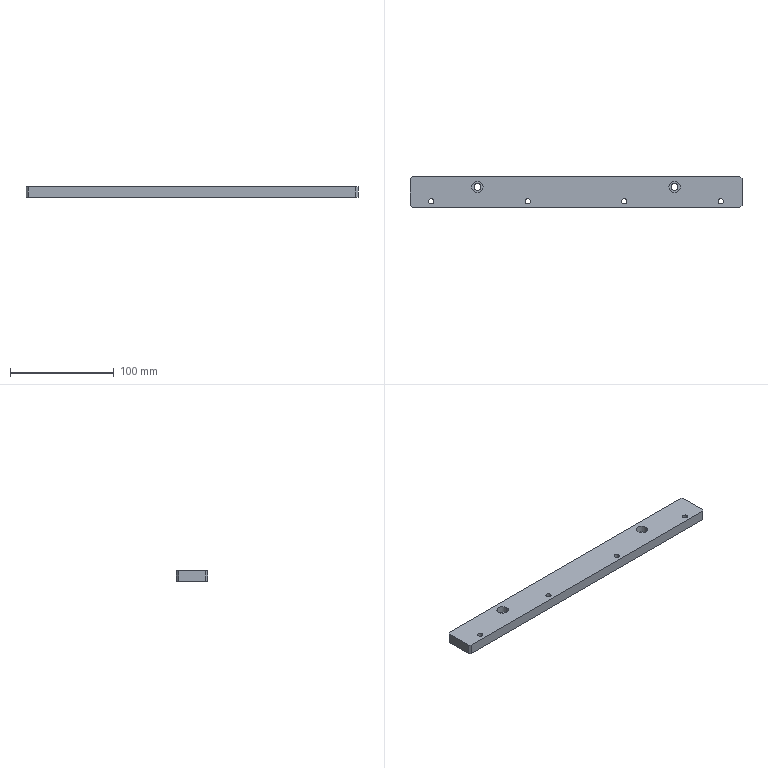Part | SolidWorks | features HoleWzd 2, Chamfer 1, Extrusion 1 | 1 solid | 28 faces | box 320 x 30 x 10 mm | volume 93623 mm3 | cylinder 16 | plane 12 | commonest cylinder face diameters 5 x8 6.6 x4 11 x4
STEP:
#1=CARTESIAN_POINT('',(-100.5,5.,3.2));
#2=VERTEX_POINT('',#1);
#3=CARTESIAN_POINT('',(-89.5,5.,3.2));
#4=VERTEX_POINT('',#3);
#5=CARTESIAN_POINT('',(-95.,5.,3.2));
#6=DIRECTION('',(0.,0.,1.));
#7=DIRECTION('',(1.,0.,0.));
#8=AXIS2_PLACEMENT_3D('',#5,#6,#7);
#9=CIRCLE('',#8,5.5);
#10=EDGE_CURVE('',#2,#4,#9,.T.);
#11=ORIENTED_EDGE('',*,*,#10,.F.);
#12=CARTESIAN_POINT('',(-100.5,5.,10.));
#13=VERTEX_POINT('',#12);
#14=CARTESIAN_POINT('',(-100.5,5.,10.));
#15=DIRECTION('',(0.,0.,1.));
#16=VECTOR('',#15,1000.);
#17=LINE('',#14,#16);
#18=EDGE_CURVE('',#2,#13,#17,.T.);
#19=ORIENTED_EDGE('',*,*,#18,.T.);
#20=CARTESIAN_POINT('',(-89.5,5.,10.));
#21=VERTEX_POINT('',#20);
#22=CARTESIAN_POINT('',(-95.,5.,10.));
#23=DIRECTION('',(0.,0.,1.));
#24=DIRECTION('',(1.,0.,0.));
#25=AXIS2_PLACEMENT_3D('',#22,#23,#24);
#26=CIRCLE('',#25,5.5);
#27=EDGE_CURVE('',#13,#21,#26,.T.);
#28=ORIENTED_EDGE('',*,*,#27,.T.);
#29=CARTESIAN_POINT('',(-89.5,5.,10.));
#30=DIRECTION('',(0.,0.,1.));
#31=VECTOR('',#30,1000.);
#32=LINE('',#29,#31);
#33=EDGE_CURVE('',#4,#21,#32,.T.);
#34=ORIENTED_EDGE('',*,*,#33,.F.);
#35=EDGE_LOOP('',(#11,#19,#28,#34));
#36=FACE_OUTER_BOUND('',#35,.T.);
#37=CARTESIAN_POINT('',(-95.,5.,10.));
#38=DIRECTION('',(0.,0.,1.));
#39=DIRECTION('',(1.,0.,0.));
#40=AXIS2_PLACEMENT_3D('',#37,#38,#39);
#41=CYLINDRICAL_SURFACE('',#40,5.5);
#42=ADVANCED_FACE('',(#36),#41,.F.);
#43=CARTESIAN_POINT('',(-98.3,5.,0.));
#44=VERTEX_POINT('',#43);
#45=CARTESIAN_POINT('',(-91.7,5.,0.));
#46=VERTEX_POINT('',#45);
#47=CARTESIAN_POINT('',(-95.,5.,0.));
#48=DIRECTION('',(0.,0.,1.));
#49=DIRECTION('',(1.,0.,0.));
#50=AXIS2_PLACEMENT_3D('',#47,#48,#49);
#51=CIRCLE('',#50,3.3);
#52=EDGE_CURVE('',#44,#46,#51,.T.);
#53=ORIENTED_EDGE('',*,*,#52,.F.);
#54=CARTESIAN_POINT('',(-98.3,5.,3.2));
#55=VERTEX_POINT('',#54);
#56=CARTESIAN_POINT('',(-98.3,5.,10.));
#57=DIRECTION('',(0.,0.,1.));
#58=VECTOR('',#57,1000.);
#59=LINE('',#56,#58);
#60=EDGE_CURVE('',#44,#55,#59,.T.);
#61=ORIENTED_EDGE('',*,*,#60,.T.);
#62=CARTESIAN_POINT('',(-91.7,5.,3.2));
#63=VERTEX_POINT('',#62);
#64=CARTESIAN_POINT('',(-95.,5.,3.2));
#65=DIRECTION('',(0.,0.,1.));
#66=DIRECTION('',(1.,0.,0.));
#67=AXIS2_PLACEMENT_3D('',#64,#65,#66);
#68=CIRCLE('',#67,3.3);
#69=EDGE_CURVE('',#55,#63,#68,.T.);
#70=ORIENTED_EDGE('',*,*,#69,.T.);
#71=CARTESIAN_POINT('',(-91.7,5.,10.));
#72=DIRECTION('',(0.,0.,1.));
#73=VECTOR('',#72,1000.);
#74=LINE('',#71,#73);
#75=EDGE_CURVE('',#46,#63,#74,.T.);
#76=ORIENTED_EDGE('',*,*,#75,.F.);
#77=EDGE_LOOP('',(#53,#61,#70,#76));
#78=FACE_OUTER_BOUND('',#77,.T.);
#79=CARTESIAN_POINT('',(-95.,5.,10.));
#80=DIRECTION('',(0.,0.,1.));
#81=DIRECTION('',(1.,0.,0.));
#82=AXIS2_PLACEMENT_3D('',#79,#80,#81);
#83=CYLINDRICAL_SURFACE('',#82,3.3);
#84=ADVANCED_FACE('',(#78),#83,.F.);
#85=CARTESIAN_POINT('',(89.5,5.,3.2));
#86=VERTEX_POINT('',#85);
#87=CARTESIAN_POINT('',(100.5,5.,3.2));
#88=VERTEX_POINT('',#87);
#89=CARTESIAN_POINT('',(95.,5.,3.2));
#90=DIRECTION('',(0.,0.,1.));
#91=DIRECTION('',(1.,0.,0.));
#92=AXIS2_PLACEMENT_3D('',#89,#90,#91);
#93=CIRCLE('',#92,5.5);
#94=EDGE_CURVE('',#86,#88,#93,.T.);
#95=ORIENTED_EDGE('',*,*,#94,.F.);
#96=CARTESIAN_POINT('',(89.5,5.,10.));
#97=VERTEX_POINT('',#96);
#98=CARTESIAN_POINT('',(89.5,5.,10.));
#99=DIRECTION('',(0.,0.,1.));
#100=VECTOR('',#99,1000.);
#101=LINE('',#98,#100);
#102=EDGE_CURVE('',#86,#97,#101,.T.);
#103=ORIENTED_EDGE('',*,*,#102,.T.);
#104=CARTESIAN_POINT('',(100.5,5.,10.));
#105=VERTEX_POINT('',#104);
#106=CARTESIAN_POINT('',(95.,5.,10.));
#107=DIRECTION('',(0.,0.,1.));
#108=DIRECTION('',(1.,0.,0.));
#109=AXIS2_PLACEMENT_3D('',#106,#107,#108);
#110=CIRCLE('',#109,5.5);
#111=EDGE_CURVE('',#97,#105,#110,.T.);
#112=ORIENTED_EDGE('',*,*,#111,.T.);
#113=CARTESIAN_POINT('',(100.5,5.,10.));
#114=DIRECTION('',(0.,0.,1.));
#115=VECTOR('',#114,1000.);
#116=LINE('',#113,#115);
#117=EDGE_CURVE('',#88,#105,#116,.T.);
#118=ORIENTED_EDGE('',*,*,#117,.F.);
#119=EDGE_LOOP('',(#95,#103,#112,#118));
#120=FACE_OUTER_BOUND('',#119,.T.);
#121=CARTESIAN_POINT('',(95.,5.,10.));
#122=DIRECTION('',(0.,0.,1.));
#123=DIRECTION('',(1.,0.,0.));
#124=AXIS2_PLACEMENT_3D('',#121,#122,#123);
#125=CYLINDRICAL_SURFACE('',#124,5.5);
#126=ADVANCED_FACE('',(#120),#125,.F.);
#127=CARTESIAN_POINT('',(91.7,5.,0.));
#128=VERTEX_POINT('',#127);
#129=CARTESIAN_POINT('',(98.3,5.,0.));
#130=VERTEX_POINT('',#129);
#131=CARTESIAN_POINT('',(95.,5.,0.));
#132=DIRECTION('',(0.,0.,1.));
#133=DIRECTION('',(1.,0.,0.));
#134=AXIS2_PLACEMENT_3D('',#131,#132,#133);
#135=CIRCLE('',#134,3.3);
#136=EDGE_CURVE('',#128,#130,#135,.T.);
#137=ORIENTED_EDGE('',*,*,#136,.F.);
#138=CARTESIAN_POINT('',(91.7,5.,3.2));
#139=VERTEX_POINT('',#138);
#140=CARTESIAN_POINT('',(91.7,5.,10.));
#141=DIRECTION('',(0.,0.,1.));
#142=VECTOR('',#141,1000.);
#143=LINE('',#140,#142);
#144=EDGE_CURVE('',#128,#139,#143,.T.);
#145=ORIENTED_EDGE('',*,*,#144,.T.);
#146=CARTESIAN_POINT('',(98.3,5.,3.2));
#147=VERTEX_POINT('',#146);
#148=CARTESIAN_POINT('',(95.,5.,3.2));
#149=DIRECTION('',(0.,0.,1.));
#150=DIRECTION('',(1.,0.,0.));
#151=AXIS2_PLACEMENT_3D('',#148,#149,#150);
#152=CIRCLE('',#151,3.3);
#153=EDGE_CURVE('',#139,#147,#152,.T.);
#154=ORIENTED_EDGE('',*,*,#153,.T.);
#155=CARTESIAN_POINT('',(98.3,5.,10.));
#156=DIRECTION('',(0.,0.,1.));
#157=VECTOR('',#156,1000.);
#158=LINE('',#155,#157);
#159=EDGE_CURVE('',#130,#147,#158,.T.);
#160=ORIENTED_EDGE('',*,*,#159,.F.);
#161=EDGE_LOOP('',(#137,#145,#154,#160));
#162=FACE_OUTER_BOUND('',#161,.T.);
#163=CARTESIAN_POINT('',(95.,5.,10.));
#164=DIRECTION('',(0.,0.,1.));
#165=DIRECTION('',(1.,0.,0.));
#166=AXIS2_PLACEMENT_3D('',#163,#164,#165);
#167=CYLINDRICAL_SURFACE('',#166,3.3);
#168=ADVANCED_FACE('',(#162),#167,.F.);
#169=CARTESIAN_POINT('',(-142.,-9.,0.));
#170=VERTEX_POINT('',#169);
#171=CARTESIAN_POINT('',(-137.,-9.,0.));
#172=VERTEX_POINT('',#171);
#173=CARTESIAN_POINT('',(-139.5,-9.,0.));
#174=DIRECTION('',(0.,0.,1.));
#175=DIRECTION('',(1.,0.,0.));
#176=AXIS2_PLACEMENT_3D('',#173,#174,#175);
#177=CIRCLE('',#176,2.5);
#178=EDGE_CURVE('',#170,#172,#177,.T.);
#179=ORIENTED_EDGE('',*,*,#178,.F.);
#180=CARTESIAN_POINT('',(-142.,-9.,10.));
#181=VERTEX_POINT('',#180);
#182=CARTESIAN_POINT('',(-142.,-9.,10.));
#183=DIRECTION('',(0.,0.,1.));
#184=VECTOR('',#183,1000.);
#185=LINE('',#182,#184);
#186=EDGE_CURVE('',#170,#181,#185,.T.);
#187=ORIENTED_EDGE('',*,*,#186,.T.);
#188=CARTESIAN_POINT('',(-137.,-9.,10.));
#189=VERTEX_POINT('',#188);
#190=CARTESIAN_POINT('',(-139.5,-9.,10.));
#191=DIRECTION('',(0.,0.,1.));
#192=DIRECTION('',(1.,0.,0.));
#193=AXIS2_PLACEMENT_3D('',#190,#191,#192);
#194=CIRCLE('',#193,2.5);
#195=EDGE_CURVE('',#181,#189,#194,.T.);
#196=ORIENTED_EDGE('',*,*,#195,.T.);
#197=CARTESIAN_POINT('',(-137.,-9.,10.));
#198=DIRECTION('',(0.,0.,1.));
#199=VECTOR('',#198,1000.);
#200=LINE('',#197,#199);
#201=EDGE_CURVE('',#172,#189,#200,.T.);
#202=ORIENTED_EDGE('',*,*,#201,.F.);
#203=EDGE_LOOP('',(#179,#187,#196,#202));
#204=FACE_OUTER_BOUND('',#203,.T.);
#205=CARTESIAN_POINT('',(-139.5,-9.,10.));
#206=DIRECTION('',(0.,0.,1.));
#207=DIRECTION('',(1.,0.,0.));
#208=AXIS2_PLACEMENT_3D('',#205,#206,#207);
#209=CYLINDRICAL_SURFACE('',#208,2.5);
#210=ADVANCED_FACE('',(#204),#209,.F.);
#211=CARTESIAN_POINT('',(-49.,-9.,0.));
#212=VERTEX_POINT('',#211);
#213=CARTESIAN_POINT('',(-44.,-9.,0.));
#214=VERTEX_POINT('',#213);
#215=CARTESIAN_POINT('',(-46.5,-9.,0.));
#216=DIRECTION('',(0.,0.,1.));
#217=DIRECTION('',(1.,0.,0.));
#218=AXIS2_PLACEMENT_3D('',#215,#216,#217);
#219=CIRCLE('',#218,2.5);
#220=EDGE_CURVE('',#212,#214,#219,.T.);
#221=ORIENTED_EDGE('',*,*,#220,.F.);
#222=CARTESIAN_POINT('',(-49.,-9.,10.));
#223=VERTEX_POINT('',#222);
#224=CARTESIAN_POINT('',(-49.,-9.,10.));
#225=DIRECTION('',(0.,0.,1.));
#226=VECTOR('',#225,1000.);
#227=LINE('',#224,#226);
#228=EDGE_CURVE('',#212,#223,#227,.T.);
#229=ORIENTED_EDGE('',*,*,#228,.T.);
#230=CARTESIAN_POINT('',(-44.,-9.,10.));
#231=VERTEX_POINT('',#230);
#232=CARTESIAN_POINT('',(-46.5,-9.,10.));
#233=DIRECTION('',(0.,0.,1.));
#234=DIRECTION('',(1.,0.,0.));
#235=AXIS2_PLACEMENT_3D('',#232,#233,#234);
#236=CIRCLE('',#235,2.5);
#237=EDGE_CURVE('',#223,#231,#236,.T.);
#238=ORIENTED_EDGE('',*,*,#237,.T.);
#239=CARTESIAN_POINT('',(-44.,-9.,10.));
#240=DIRECTION('',(0.,0.,1.));
#241=VECTOR('',#240,1000.);
#242=LINE('',#239,#241);
#243=EDGE_CURVE('',#214,#231,#242,.T.);
#244=ORIENTED_EDGE('',*,*,#243,.F.);
#245=EDGE_LOOP('',(#221,#229,#238,#244));
#246=FACE_OUTER_BOUND('',#245,.T.);
#247=CARTESIAN_POINT('',(-46.5,-9.,10.));
#248=DIRECTION('',(0.,0.,1.));
#249=DIRECTION('',(1.,0.,0.));
#250=AXIS2_PLACEMENT_3D('',#247,#248,#249);
#251=CYLINDRICAL_SURFACE('',#250,2.5);
#252=ADVANCED_FACE('',(#246),#251,.F.);
#253=CARTESIAN_POINT('',(44.,-9.,0.));
#254=VERTEX_POINT('',#253);
#255=CARTESIAN_POINT('',(49.,-9.,0.));
#256=VERTEX_POINT('',#255);
#257=CARTESIAN_POINT('',(46.5,-9.,0.));
#258=DIRECTION('',(0.,0.,1.));
#259=DIRECTION('',(1.,0.,0.));
#260=AXIS2_PLACEMENT_3D('',#257,#258,#259);
#261=CIRCLE('',#260,2.5);
#262=EDGE_CURVE('',#254,#256,#261,.T.);
#263=ORIENTED_EDGE('',*,*,#262,.F.);
#264=CARTESIAN_POINT('',(44.,-9.,10.));
#265=VERTEX_POINT('',#264);
#266=CARTESIAN_POINT('',(44.,-9.,10.));
#267=DIRECTION('',(0.,0.,1.));
#268=VECTOR('',#267,1000.);
#269=LINE('',#266,#268);
#270=EDGE_CURVE('',#254,#265,#269,.T.);
#271=ORIENTED_EDGE('',*,*,#270,.T.);
#272=CARTESIAN_POINT('',(49.,-9.,10.));
#273=VERTEX_POINT('',#272);
#274=CARTESIAN_POINT('',(46.5,-9.,10.));
#275=DIRECTION('',(0.,0.,1.));
#276=DIRECTION('',(1.,0.,0.));
#277=AXIS2_PLACEMENT_3D('',#274,#275,#276);
#278=CIRCLE('',#277,2.5);
#279=EDGE_CURVE('',#265,#273,#278,.T.);
#280=ORIENTED_EDGE('',*,*,#279,.T.);
#281=CARTESIAN_POINT('',(49.,-9.,10.));
#282=DIRECTION('',(0.,0.,1.));
#283=VECTOR('',#282,1000.);
#284=LINE('',#281,#283);
#285=EDGE_CURVE('',#256,#273,#284,.T.);
#286=ORIENTED_EDGE('',*,*,#285,.F.);
#287=EDGE_LOOP('',(#263,#271,#280,#286));
#288=FACE_OUTER_BOUND('',#287,.T.);
#289=CARTESIAN_POINT('',(46.5,-9.,10.));
#290=DIRECTION('',(0.,0.,1.));
#291=DIRECTION('',(1.,0.,0.));
#292=AXIS2_PLACEMENT_3D('',#289,#290,#291);
#293=CYLINDRICAL_SURFACE('',#292,2.5);
#294=ADVANCED_FACE('',(#288),#293,.F.);
#295=CARTESIAN_POINT('',(137.,-9.,0.));
#296=VERTEX_POINT('',#295);
#297=CARTESIAN_POINT('',(142.,-9.,0.));
#298=VERTEX_POINT('',#297);
#299=CARTESIAN_POINT('',(139.5,-9.,0.));
#300=DIRECTION('',(0.,0.,1.));
#301=DIRECTION('',(1.,0.,0.));
#302=AXIS2_PLACEMENT_3D('',#299,#300,#301);
#303=CIRCLE('',#302,2.5);
#304=EDGE_CURVE('',#296,#298,#303,.T.);
#305=ORIENTED_EDGE('',*,*,#304,.F.);
#306=CARTESIAN_POINT('',(137.,-9.,10.));
#307=VERTEX_POINT('',#306);
#308=CARTESIAN_POINT('',(137.,-9.,10.));
#309=DIRECTION('',(0.,0.,1.));
#310=VECTOR('',#309,1000.);
#311=LINE('',#308,#310);
#312=EDGE_CURVE('',#296,#307,#311,.T.);
#313=ORIENTED_EDGE('',*,*,#312,.T.);
#314=CARTESIAN_POINT('',(142.,-9.,10.));
#315=VERTEX_POINT('',#314);
#316=CARTESIAN_POINT('',(139.5,-9.,10.));
#317=DIRECTION('',(0.,0.,1.));
#318=DIRECTION('',(1.,0.,0.));
#319=AXIS2_PLACEMENT_3D('',#316,#317,#318);
#320=CIRCLE('',#319,2.5);
#321=EDGE_CURVE('',#307,#315,#320,.T.);
#322=ORIENTED_EDGE('',*,*,#321,.T.);
#323=CARTESIAN_POINT('',(142.,-9.,10.));
#324=DIRECTION('',(0.,0.,1.));
#325=VECTOR('',#324,1000.);
#326=LINE('',#323,#325);
#327=EDGE_CURVE('',#298,#315,#326,.T.);
#328=ORIENTED_EDGE('',*,*,#327,.F.);
#329=EDGE_LOOP('',(#305,#313,#322,#328));
#330=FACE_OUTER_BOUND('',#329,.T.);
#331=CARTESIAN_POINT('',(139.5,-9.,10.));
#332=DIRECTION('',(0.,0.,1.));
#333=DIRECTION('',(1.,0.,0.));
#334=AXIS2_PLACEMENT_3D('',#331,#332,#333);
#335=CYLINDRICAL_SURFACE('',#334,2.5);
#336=ADVANCED_FACE('',(#330),#335,.F.);
#337=CARTESIAN_POINT('',(160.,-13.,10.));
#338=VERTEX_POINT('',#337);
#339=CARTESIAN_POINT('',(160.,13.,10.));
#340=VERTEX_POINT('',#339);
#341=CARTESIAN_POINT('',(160.,-15.,10.));
#342=DIRECTION('',(0.,1.,0.));
#343=VECTOR('',#342,1000.);
#344=LINE('',#341,#343);
#345=EDGE_CURVE('',#338,#340,#344,.T.);
#346=ORIENTED_EDGE('',*,*,#345,.F.);
#347=CARTESIAN_POINT('',(160.,-13.,0.));
#348=VERTEX_POINT('',#347);
#349=CARTESIAN_POINT('',(160.,-13.,10.));
#350=DIRECTION('',(0.,0.,-1.));
#351=VECTOR('',#350,1000.);
#352=LINE('',#349,#351);
#353=EDGE_CURVE('',#338,#348,#352,.T.);
#354=ORIENTED_EDGE('',*,*,#353,.T.);
#355=CARTESIAN_POINT('',(160.,13.,0.));
#356=VERTEX_POINT('',#355);
#357=CARTESIAN_POINT('',(160.,-15.,0.));
#358=DIRECTION('',(0.,1.,0.));
#359=VECTOR('',#358,1000.);
#360=LINE('',#357,#359);
#361=EDGE_CURVE('',#348,#356,#360,.T.);
#362=ORIENTED_EDGE('',*,*,#361,.T.);
#363=CARTESIAN_POINT('',(160.,13.,10.));
#364=DIRECTION('',(0.,0.,1.));
#365=VECTOR('',#364,1000.);
#366=LINE('',#363,#365);
#367=EDGE_CURVE('',#356,#340,#366,.T.);
#368=ORIENTED_EDGE('',*,*,#367,.T.);
#369=EDGE_LOOP('',(#346,#354,#362,#368));
#370=FACE_OUTER_BOUND('',#369,.T.);
#371=CARTESIAN_POINT('',(160.,-15.,10.));
#372=DIRECTION('',(-1.,0.,0.));
#373=DIRECTION('',(0.,0.,1.));
#374=AXIS2_PLACEMENT_3D('',#371,#372,#373);
#375=PLANE('',#374);
#376=ADVANCED_FACE('',(#370),#375,.F.);
#377=CARTESIAN_POINT('',(158.,15.,10.));
#378=VERTEX_POINT('',#377);
#379=CARTESIAN_POINT('',(-158.,15.,10.));
#380=VERTEX_POINT('',#379);
#381=CARTESIAN_POINT('',(-160.,15.,10.));
#382=DIRECTION('',(-1.,0.,0.));
#383=VECTOR('',#382,1000.);
#384=LINE('',#381,#383);
#385=EDGE_CURVE('',#378,#380,#384,.T.);
#386=ORIENTED_EDGE('',*,*,#385,.F.);
#387=CARTESIAN_POINT('',(158.,15.,0.));
#388=VERTEX_POINT('',#387);
#389=CARTESIAN_POINT('',(158.,15.,10.));
#390=DIRECTION('',(0.,0.,-1.));
#391=VECTOR('',#390,1000.);
#392=LINE('',#389,#391);
#393=EDGE_CURVE('',#378,#388,#392,.T.);
#394=ORIENTED_EDGE('',*,*,#393,.T.);
#395=CARTESIAN_POINT('',(-158.,15.,0.));
#396=VERTEX_POINT('',#395);
#397=CARTESIAN_POINT('',(-160.,15.,0.));
#398=DIRECTION('',(-1.,0.,0.));
#399=VECTOR('',#398,1000.);
#400=LINE('',#397,#399);
#401=EDGE_CURVE('',#388,#396,#400,.T.);
#402=ORIENTED_EDGE('',*,*,#401,.T.);
#403=CARTESIAN_POINT('',(-158.,15.,10.));
#404=DIRECTION('',(0.,0.,1.));
#405=VECTOR('',#404,1000.);
#406=LINE('',#403,#405);
#407=EDGE_CURVE('',#396,#380,#406,.T.);
#408=ORIENTED_EDGE('',*,*,#407,.T.);
#409=EDGE_LOOP('',(#386,#394,#402,#408));
#410=FACE_OUTER_BOUND('',#409,.T.);
#411=CARTESIAN_POINT('',(-160.,15.,10.));
#412=DIRECTION('',(0.,-1.,0.));
#413=DIRECTION('',(0.,0.,-1.));
#414=AXIS2_PLACEMENT_3D('',#411,#412,#413);
#415=PLANE('',#414);
#416=ADVANCED_FACE('',(#410),#415,.F.);
#417=CARTESIAN_POINT('',(-160.,13.,0.));
#418=VERTEX_POINT('',#417);
#419=CARTESIAN_POINT('',(-160.,-13.,0.));
#420=VERTEX_POINT('',#419);
#421=CARTESIAN_POINT('',(-160.,-15.,0.));
#422=DIRECTION('',(0.,-1.,0.));
#423=VECTOR('',#422,1000.);
#424=LINE('',#421,#423);
#425=EDGE_CURVE('',#418,#420,#424,.T.);
#426=ORIENTED_EDGE('',*,*,#425,.T.);
#427=CARTESIAN_POINT('',(-160.,-13.,10.));
#428=VERTEX_POINT('',#427);
#429=CARTESIAN_POINT('',(-160.,-13.,10.));
#430=DIRECTION('',(0.,0.,1.));
#431=VECTOR('',#430,1000.);
#432=LINE('',#429,#431);
#433=EDGE_CURVE('',#420,#428,#432,.T.);
#434=ORIENTED_EDGE('',*,*,#433,.T.);
#435=CARTESIAN_POINT('',(-160.,13.,10.));
#436=VERTEX_POINT('',#435);
#437=CARTESIAN_POINT('',(-160.,-15.,10.));
#438=DIRECTION('',(0.,-1.,0.));
#439=VECTOR('',#438,1000.);
#440=LINE('',#437,#439);
#441=EDGE_CURVE('',#436,#428,#440,.T.);
#442=ORIENTED_EDGE('',*,*,#441,.F.);
#443=CARTESIAN_POINT('',(-160.,13.,10.));
#444=DIRECTION('',(0.,0.,-1.));
#445=VECTOR('',#444,1000.);
#446=LINE('',#443,#445);
#447=EDGE_CURVE('',#436,#418,#446,.T.);
#448=ORIENTED_EDGE('',*,*,#447,.T.);
#449=EDGE_LOOP('',(#426,#434,#442,#448));
#450=FACE_OUTER_BOUND('',#449,.T.);
#451=CARTESIAN_POINT('',(-160.,-15.,10.));
#452=DIRECTION('',(1.,0.,0.));
#453=DIRECTION('',(0.,0.,-1.));
#454=AXIS2_PLACEMENT_3D('',#451,#452,#453);
#455=PLANE('',#454);
#456=ADVANCED_FACE('',(#450),#455,.F.);
#457=CARTESIAN_POINT('',(-158.,-15.,0.));
#458=VERTEX_POINT('',#457);
#459=CARTESIAN_POINT('',(158.,-15.,0.));
#460=VERTEX_POINT('',#459);
#461=CARTESIAN_POINT('',(-160.,-15.,0.));
#462=DIRECTION('',(1.,0.,0.));
#463=VECTOR('',#462,1000.);
#464=LINE('',#461,#463);
#465=EDGE_CURVE('',#458,#460,#464,.T.);
#466=ORIENTED_EDGE('',*,*,#465,.T.);
#467=CARTESIAN_POINT('',(158.,-15.,10.));
#468=VERTEX_POINT('',#467);
#469=CARTESIAN_POINT('',(158.,-15.,10.));
#470=DIRECTION('',(0.,0.,1.));
#471=VECTOR('',#470,1000.);
#472=LINE('',#469,#471);
#473=EDGE_CURVE('',#460,#468,#472,.T.);
#474=ORIENTED_EDGE('',*,*,#473,.T.);
#475=CARTESIAN_POINT('',(-158.,-15.,10.));
#476=VERTEX_POINT('',#475);
#477=CARTESIAN_POINT('',(-160.,-15.,10.));
#478=DIRECTION('',(1.,0.,0.));
#479=VECTOR('',#478,1000.);
#480=LINE('',#477,#479);
#481=EDGE_CURVE('',#476,#468,#480,.T.);
#482=ORIENTED_EDGE('',*,*,#481,.F.);
#483=CARTESIAN_POINT('',(-158.,-15.,10.));
#484=DIRECTION('',(0.,0.,-1.));
#485=VECTOR('',#484,1000.);
#486=LINE('',#483,#485);
#487=EDGE_CURVE('',#476,#458,#486,.T.);
#488=ORIENTED_EDGE('',*,*,#487,.T.);
#489=EDGE_LOOP('',(#466,#474,#482,#488));
#490=FACE_OUTER_BOUND('',#489,.T.);
#491=CARTESIAN_POINT('',(-160.,-15.,10.));
#492=DIRECTION('',(0.,1.,0.));
#493=DIRECTION('',(0.,0.,1.));
#494=AXIS2_PLACEMENT_3D('',#491,#492,#493);
#495=PLANE('',#494);
#496=ADVANCED_FACE('',(#490),#495,.F.);
#497=CARTESIAN_POINT('',(-95.,5.,10.));
#498=DIRECTION('',(0.,0.,1.));
#499=DIRECTION('',(1.,0.,0.));
#500=AXIS2_PLACEMENT_3D('',#497,#498,#499);
#501=CIRCLE('',#500,5.5);
#502=EDGE_CURVE('',#21,#13,#501,.T.);
#503=ORIENTED_EDGE('',*,*,#502,.F.);
#504=ORIENTED_EDGE('',*,*,#27,.F.);
#505=EDGE_LOOP('',(#503,#504));
#506=FACE_BOUND('',#505,.T.);
#507=CARTESIAN_POINT('',(95.,5.,10.));
#508=DIRECTION('',(0.,0.,1.));
#509=DIRECTION('',(1.,0.,0.));
#510=AXIS2_PLACEMENT_3D('',#507,#508,#509);
#511=CIRCLE('',#510,5.5);
#512=EDGE_CURVE('',#105,#97,#511,.T.);
#513=ORIENTED_EDGE('',*,*,#512,.F.);
#514=ORIENTED_EDGE('',*,*,#111,.F.);
#515=EDGE_LOOP('',(#513,#514));
#516=FACE_BOUND('',#515,.T.);
#517=CARTESIAN_POINT('',(-139.5,-9.,10.));
#518=DIRECTION('',(0.,0.,1.));
#519=DIRECTION('',(1.,0.,0.));
#520=AXIS2_PLACEMENT_3D('',#517,#518,#519);
#521=CIRCLE('',#520,2.5);
#522=EDGE_CURVE('',#189,#181,#521,.T.);
#523=ORIENTED_EDGE('',*,*,#522,.F.);
#524=ORIENTED_EDGE('',*,*,#195,.F.);
#525=EDGE_LOOP('',(#523,#524));
#526=FACE_BOUND('',#525,.T.);
#527=CARTESIAN_POINT('',(-46.5,-9.,10.));
#528=DIRECTION('',(0.,0.,1.));
#529=DIRECTION('',(1.,0.,0.));
#530=AXIS2_PLACEMENT_3D('',#527,#528,#529);
#531=CIRCLE('',#530,2.5);
#532=EDGE_CURVE('',#231,#223,#531,.T.);
#533=ORIENTED_EDGE('',*,*,#532,.F.);
#534=ORIENTED_EDGE('',*,*,#237,.F.);
#535=EDGE_LOOP('',(#533,#534));
#536=FACE_BOUND('',#535,.T.);
#537=CARTESIAN_POINT('',(46.5,-9.,10.));
#538=DIRECTION('',(0.,0.,1.));
#539=DIRECTION('',(1.,0.,0.));
#540=AXIS2_PLACEMENT_3D('',#537,#538,#539);
#541=CIRCLE('',#540,2.5);
#542=EDGE_CURVE('',#273,#265,#541,.T.);
#543=ORIENTED_EDGE('',*,*,#542,.F.);
#544=ORIENTED_EDGE('',*,*,#279,.F.);
#545=EDGE_LOOP('',(#543,#544));
#546=FACE_BOUND('',#545,.T.);
#547=CARTESIAN_POINT('',(139.5,-9.,10.));
#548=DIRECTION('',(0.,0.,1.));
#549=DIRECTION('',(1.,0.,0.));
#550=AXIS2_PLACEMENT_3D('',#547,#548,#549);
#551=CIRCLE('',#550,2.5);
#552=EDGE_CURVE('',#315,#307,#551,.T.);
#553=ORIENTED_EDGE('',*,*,#552,.F.);
#554=ORIENTED_EDGE('',*,*,#321,.F.);
#555=EDGE_LOOP('',(#553,#554));
#556=FACE_BOUND('',#555,.T.);
#557=ORIENTED_EDGE('',*,*,#481,.T.);
#558=CARTESIAN_POINT('',(160.,-13.,10.));
#559=DIRECTION('',(0.7071,0.7071,0.));
#560=VECTOR('',#559,1000.);
#561=LINE('',#558,#560);
#562=EDGE_CURVE('',#468,#338,#561,.T.);
#563=ORIENTED_EDGE('',*,*,#562,.T.);
#564=ORIENTED_EDGE('',*,*,#345,.T.);
#565=CARTESIAN_POINT('',(158.,15.,10.));
#566=DIRECTION('',(-0.7071,0.7071,0.));
#567=VECTOR('',#566,1000.);
#568=LINE('',#565,#567);
#569=EDGE_CURVE('',#340,#378,#568,.T.);
#570=ORIENTED_EDGE('',*,*,#569,.T.);
#571=ORIENTED_EDGE('',*,*,#385,.T.);
#572=CARTESIAN_POINT('',(-160.,13.,10.));
#573=DIRECTION('',(-0.7071,-0.7071,0.));
#574=VECTOR('',#573,1000.);
#575=LINE('',#572,#574);
#576=EDGE_CURVE('',#380,#436,#575,.T.);
#577=ORIENTED_EDGE('',*,*,#576,.T.);
#578=ORIENTED_EDGE('',*,*,#441,.T.);
#579=CARTESIAN_POINT('',(-158.,-15.,10.));
#580=DIRECTION('',(0.7071,-0.7071,0.));
#581=VECTOR('',#580,1000.);
#582=LINE('',#579,#581);
#583=EDGE_CURVE('',#428,#476,#582,.T.);
#584=ORIENTED_EDGE('',*,*,#583,.T.);
#585=EDGE_LOOP('',(#557,#563,#564,#570,#571,#577,#578,#584));
#586=FACE_OUTER_BOUND('',#585,.T.);
#587=CARTESIAN_POINT('',(0.,0.,10.));
#588=DIRECTION('',(0.,0.,-1.));
#589=DIRECTION('',(-1.,0.,0.));
#590=AXIS2_PLACEMENT_3D('',#587,#588,#589);
#591=PLANE('',#590);
#592=ADVANCED_FACE('',(#506,#516,#526,#536,#546,#556,#586),#591,.F.);
#593=CARTESIAN_POINT('',(-95.,5.,0.));
#594=DIRECTION('',(0.,0.,1.));
#595=DIRECTION('',(1.,0.,0.));
#596=AXIS2_PLACEMENT_3D('',#593,#594,#595);
#597=CIRCLE('',#596,3.3);
#598=EDGE_CURVE('',#46,#44,#597,.T.);
#599=ORIENTED_EDGE('',*,*,#598,.T.);
#600=ORIENTED_EDGE('',*,*,#52,.T.);
#601=EDGE_LOOP('',(#599,#600));
#602=FACE_BOUND('',#601,.T.);
#603=CARTESIAN_POINT('',(95.,5.,0.));
#604=DIRECTION('',(0.,0.,1.));
#605=DIRECTION('',(1.,0.,0.));
#606=AXIS2_PLACEMENT_3D('',#603,#604,#605);
#607=CIRCLE('',#606,3.3);
#608=EDGE_CURVE('',#130,#128,#607,.T.);
#609=ORIENTED_EDGE('',*,*,#608,.T.);
#610=ORIENTED_EDGE('',*,*,#136,.T.);
#611=EDGE_LOOP('',(#609,#610));
#612=FACE_BOUND('',#611,.T.);
#613=CARTESIAN_POINT('',(-139.5,-9.,0.));
#614=DIRECTION('',(0.,0.,1.));
#615=DIRECTION('',(1.,0.,0.));
#616=AXIS2_PLACEMENT_3D('',#613,#614,#615);
#617=CIRCLE('',#616,2.5);
#618=EDGE_CURVE('',#172,#170,#617,.T.);
#619=ORIENTED_EDGE('',*,*,#618,.T.);
#620=ORIENTED_EDGE('',*,*,#178,.T.);
#621=EDGE_LOOP('',(#619,#620));
#622=FACE_BOUND('',#621,.T.);
#623=CARTESIAN_POINT('',(-46.5,-9.,0.));
#624=DIRECTION('',(0.,0.,1.));
#625=DIRECTION('',(1.,0.,0.));
#626=AXIS2_PLACEMENT_3D('',#623,#624,#625);
#627=CIRCLE('',#626,2.5);
#628=EDGE_CURVE('',#214,#212,#627,.T.);
#629=ORIENTED_EDGE('',*,*,#628,.T.);
#630=ORIENTED_EDGE('',*,*,#220,.T.);
#631=EDGE_LOOP('',(#629,#630));
#632=FACE_BOUND('',#631,.T.);
#633=CARTESIAN_POINT('',(46.5,-9.,0.));
#634=DIRECTION('',(0.,0.,1.));
#635=DIRECTION('',(1.,0.,0.));
#636=AXIS2_PLACEMENT_3D('',#633,#634,#635);
#637=CIRCLE('',#636,2.5);
#638=EDGE_CURVE('',#256,#254,#637,.T.);
#639=ORIENTED_EDGE('',*,*,#638,.T.);
#640=ORIENTED_EDGE('',*,*,#262,.T.);
#641=EDGE_LOOP('',(#639,#640));
#642=FACE_BOUND('',#641,.T.);
#643=CARTESIAN_POINT('',(139.5,-9.,0.));
#644=DIRECTION('',(0.,0.,1.));
#645=DIRECTION('',(1.,0.,0.));
#646=AXIS2_PLACEMENT_3D('',#643,#644,#645);
#647=CIRCLE('',#646,2.5);
#648=EDGE_CURVE('',#298,#296,#647,.T.);
#649=ORIENTED_EDGE('',*,*,#648,.T.);
#650=ORIENTED_EDGE('',*,*,#304,.T.);
#651=EDGE_LOOP('',(#649,#650));
#652=FACE_BOUND('',#651,.T.);
#653=ORIENTED_EDGE('',*,*,#361,.F.);
#654=CARTESIAN_POINT('',(86.5,-86.5,0.));
#655=DIRECTION('',(-0.7071,-0.7071,0.));
#656=VECTOR('',#655,1000.);
#657=LINE('',#654,#656);
#658=EDGE_CURVE('',#348,#460,#657,.T.);
#659=ORIENTED_EDGE('',*,*,#658,.T.);
#660=ORIENTED_EDGE('',*,*,#465,.F.);
#661=CARTESIAN_POINT('',(-86.5,-86.5,0.));
#662=DIRECTION('',(-0.7071,0.7071,0.));
#663=VECTOR('',#662,1000.);
#664=LINE('',#661,#663);
#665=EDGE_CURVE('',#458,#420,#664,.T.);
#666=ORIENTED_EDGE('',*,*,#665,.T.);
#667=ORIENTED_EDGE('',*,*,#425,.F.);
#668=CARTESIAN_POINT('',(-86.5,86.5,0.));
#669=DIRECTION('',(0.7071,0.7071,0.));
#670=VECTOR('',#669,1000.);
#671=LINE('',#668,#670);
#672=EDGE_CURVE('',#418,#396,#671,.T.);
#673=ORIENTED_EDGE('',*,*,#672,.T.);
#674=ORIENTED_EDGE('',*,*,#401,.F.);
#675=CARTESIAN_POINT('',(86.5,86.5,0.));
#676=DIRECTION('',(0.7071,-0.7071,0.));
#677=VECTOR('',#676,1000.);
#678=LINE('',#675,#677);
#679=EDGE_CURVE('',#388,#356,#678,.T.);
#680=ORIENTED_EDGE('',*,*,#679,.T.);
#681=EDGE_LOOP('',(#653,#659,#660,#666,#667,#673,#674,#680));
#682=FACE_OUTER_BOUND('',#681,.T.);
#683=CARTESIAN_POINT('',(0.,0.,0.));
#684=DIRECTION('',(0.,0.,-1.));
#685=DIRECTION('',(-1.,0.,0.));
#686=AXIS2_PLACEMENT_3D('',#683,#684,#685);
#687=PLANE('',#686);
#688=ADVANCED_FACE('',(#602,#612,#622,#632,#642,#652,#682),#687,.T.);
#689=ORIENTED_EDGE('',*,*,#562,.F.);
#690=ORIENTED_EDGE('',*,*,#473,.F.);
#691=ORIENTED_EDGE('',*,*,#658,.F.);
#692=ORIENTED_EDGE('',*,*,#353,.F.);
#693=EDGE_LOOP('',(#689,#690,#691,#692));
#694=FACE_OUTER_BOUND('',#693,.T.);
#695=CARTESIAN_POINT('',(160.,-13.,10.));
#696=DIRECTION('',(-0.7071,0.7071,0.));
#697=DIRECTION('',(0.,0.,-1.));
#698=AXIS2_PLACEMENT_3D('',#695,#696,#697);
#699=PLANE('',#698);
#700=ADVANCED_FACE('',(#694),#699,.F.);
#701=ORIENTED_EDGE('',*,*,#569,.F.);
#702=ORIENTED_EDGE('',*,*,#367,.F.);
#703=ORIENTED_EDGE('',*,*,#679,.F.);
#704=ORIENTED_EDGE('',*,*,#393,.F.);
#705=EDGE_LOOP('',(#701,#702,#703,#704));
#706=FACE_OUTER_BOUND('',#705,.T.);
#707=CARTESIAN_POINT('',(158.,15.,10.));
#708=DIRECTION('',(-0.7071,-0.7071,0.));
#709=DIRECTION('',(0.,0.,-1.));
#710=AXIS2_PLACEMENT_3D('',#707,#708,#709);
#711=PLANE('',#710);
#712=ADVANCED_FACE('',(#706),#711,.F.);
#713=ORIENTED_EDGE('',*,*,#583,.F.);
#714=ORIENTED_EDGE('',*,*,#433,.F.);
#715=ORIENTED_EDGE('',*,*,#665,.F.);
#716=ORIENTED_EDGE('',*,*,#487,.F.);
#717=EDGE_LOOP('',(#713,#714,#715,#716));
#718=FACE_OUTER_BOUND('',#717,.T.);
#719=CARTESIAN_POINT('',(-158.,-15.,10.));
#720=DIRECTION('',(0.7071,0.7071,0.));
#721=DIRECTION('',(0.,0.,-1.));
#722=AXIS2_PLACEMENT_3D('',#719,#720,#721);
#723=PLANE('',#722);
#724=ADVANCED_FACE('',(#718),#723,.F.);
#725=ORIENTED_EDGE('',*,*,#576,.F.);
#726=ORIENTED_EDGE('',*,*,#407,.F.);
#727=ORIENTED_EDGE('',*,*,#672,.F.);
#728=ORIENTED_EDGE('',*,*,#447,.F.);
#729=EDGE_LOOP('',(#725,#726,#727,#728));
#730=FACE_OUTER_BOUND('',#729,.T.);
#731=CARTESIAN_POINT('',(-160.,13.,10.));
#732=DIRECTION('',(0.7071,-0.7071,0.));
#733=DIRECTION('',(0.,0.,-1.));
#734=AXIS2_PLACEMENT_3D('',#731,#732,#733);
#735=PLANE('',#734);
#736=ADVANCED_FACE('',(#730),#735,.F.);
#737=ORIENTED_EDGE('',*,*,#312,.F.);
#738=ORIENTED_EDGE('',*,*,#648,.F.);
#739=ORIENTED_EDGE('',*,*,#327,.T.);
#740=ORIENTED_EDGE('',*,*,#552,.T.);
#741=EDGE_LOOP('',(#737,#738,#739,#740));
#742=FACE_OUTER_BOUND('',#741,.T.);
#743=CARTESIAN_POINT('',(139.5,-9.,10.));
#744=DIRECTION('',(0.,0.,1.));
#745=DIRECTION('',(1.,0.,0.));
#746=AXIS2_PLACEMENT_3D('',#743,#744,#745);
#747=CYLINDRICAL_SURFACE('',#746,2.5);
#748=ADVANCED_FACE('',(#742),#747,.F.);
#749=ORIENTED_EDGE('',*,*,#270,.F.);
#750=ORIENTED_EDGE('',*,*,#638,.F.);
#751=ORIENTED_EDGE('',*,*,#285,.T.);
#752=ORIENTED_EDGE('',*,*,#542,.T.);
#753=EDGE_LOOP('',(#749,#750,#751,#752));
#754=FACE_OUTER_BOUND('',#753,.T.);
#755=CARTESIAN_POINT('',(46.5,-9.,10.));
#756=DIRECTION('',(0.,0.,1.));
#757=DIRECTION('',(1.,0.,0.));
#758=AXIS2_PLACEMENT_3D('',#755,#756,#757);
#759=CYLINDRICAL_SURFACE('',#758,2.5);
#760=ADVANCED_FACE('',(#754),#759,.F.);
#761=ORIENTED_EDGE('',*,*,#228,.F.);
#762=ORIENTED_EDGE('',*,*,#628,.F.);
#763=ORIENTED_EDGE('',*,*,#243,.T.);
#764=ORIENTED_EDGE('',*,*,#532,.T.);
#765=EDGE_LOOP('',(#761,#762,#763,#764));
#766=FACE_OUTER_BOUND('',#765,.T.);
#767=CARTESIAN_POINT('',(-46.5,-9.,10.));
#768=DIRECTION('',(0.,0.,1.));
#769=DIRECTION('',(1.,0.,0.));
#770=AXIS2_PLACEMENT_3D('',#767,#768,#769);
#771=CYLINDRICAL_SURFACE('',#770,2.5);
#772=ADVANCED_FACE('',(#766),#771,.F.);
#773=ORIENTED_EDGE('',*,*,#186,.F.);
#774=ORIENTED_EDGE('',*,*,#618,.F.);
#775=ORIENTED_EDGE('',*,*,#201,.T.);
#776=ORIENTED_EDGE('',*,*,#522,.T.);
#777=EDGE_LOOP('',(#773,#774,#775,#776));
#778=FACE_OUTER_BOUND('',#777,.T.);
#779=CARTESIAN_POINT('',(-139.5,-9.,10.));
#780=DIRECTION('',(0.,0.,1.));
#781=DIRECTION('',(1.,0.,0.));
#782=AXIS2_PLACEMENT_3D('',#779,#780,#781);
#783=CYLINDRICAL_SURFACE('',#782,2.5);
#784=ADVANCED_FACE('',(#778),#783,.F.);
#785=ORIENTED_EDGE('',*,*,#144,.F.);
#786=ORIENTED_EDGE('',*,*,#608,.F.);
#787=ORIENTED_EDGE('',*,*,#159,.T.);
#788=CARTESIAN_POINT('',(95.,5.,3.2));
#789=DIRECTION('',(0.,0.,1.));
#790=DIRECTION('',(1.,0.,0.));
#791=AXIS2_PLACEMENT_3D('',#788,#789,#790);
#792=CIRCLE('',#791,3.3);
#793=EDGE_CURVE('',#147,#139,#792,.T.);
#794=ORIENTED_EDGE('',*,*,#793,.T.);
#795=EDGE_LOOP('',(#785,#786,#787,#794));
#796=FACE_OUTER_BOUND('',#795,.T.);
#797=CARTESIAN_POINT('',(95.,5.,10.));
#798=DIRECTION('',(0.,0.,1.));
#799=DIRECTION('',(1.,0.,0.));
#800=AXIS2_PLACEMENT_3D('',#797,#798,#799);
#801=CYLINDRICAL_SURFACE('',#800,3.3);
#802=ADVANCED_FACE('',(#796),#801,.F.);
#803=ORIENTED_EDGE('',*,*,#793,.F.);
#804=ORIENTED_EDGE('',*,*,#153,.F.);
#805=EDGE_LOOP('',(#803,#804));
#806=FACE_BOUND('',#805,.T.);
#807=CARTESIAN_POINT('',(95.,5.,3.2));
#808=DIRECTION('',(0.,0.,1.));
#809=DIRECTION('',(1.,0.,0.));
#810=AXIS2_PLACEMENT_3D('',#807,#808,#809);
#811=CIRCLE('',#810,5.5);
#812=EDGE_CURVE('',#88,#86,#811,.T.);
#813=ORIENTED_EDGE('',*,*,#812,.T.);
#814=ORIENTED_EDGE('',*,*,#94,.T.);
#815=EDGE_LOOP('',(#813,#814));
#816=FACE_OUTER_BOUND('',#815,.T.);
#817=CARTESIAN_POINT('',(98.3,5.,3.2));
#818=DIRECTION('',(0.,0.,-1.));
#819=DIRECTION('',(-1.,0.,0.));
#820=AXIS2_PLACEMENT_3D('',#817,#818,#819);
#821=PLANE('',#820);
#822=ADVANCED_FACE('',(#806,#816),#821,.F.);
#823=ORIENTED_EDGE('',*,*,#102,.F.);
#824=ORIENTED_EDGE('',*,*,#812,.F.);
#825=ORIENTED_EDGE('',*,*,#117,.T.);
#826=ORIENTED_EDGE('',*,*,#512,.T.);
#827=EDGE_LOOP('',(#823,#824,#825,#826));
#828=FACE_OUTER_BOUND('',#827,.T.);
#829=CARTESIAN_POINT('',(95.,5.,10.));
#830=DIRECTION('',(0.,0.,1.));
#831=DIRECTION('',(1.,0.,0.));
#832=AXIS2_PLACEMENT_3D('',#829,#830,#831);
#833=CYLINDRICAL_SURFACE('',#832,5.5);
#834=ADVANCED_FACE('',(#828),#833,.F.);
#835=ORIENTED_EDGE('',*,*,#60,.F.);
#836=ORIENTED_EDGE('',*,*,#598,.F.);
#837=ORIENTED_EDGE('',*,*,#75,.T.);
#838=CARTESIAN_POINT('',(-95.,5.,3.2));
#839=DIRECTION('',(0.,0.,1.));
#840=DIRECTION('',(1.,0.,0.));
#841=AXIS2_PLACEMENT_3D('',#838,#839,#840);
#842=CIRCLE('',#841,3.3);
#843=EDGE_CURVE('',#63,#55,#842,.T.);
#844=ORIENTED_EDGE('',*,*,#843,.T.);
#845=EDGE_LOOP('',(#835,#836,#837,#844));
#846=FACE_OUTER_BOUND('',#845,.T.);
#847=CARTESIAN_POINT('',(-95.,5.,10.));
#848=DIRECTION('',(0.,0.,1.));
#849=DIRECTION('',(1.,0.,0.));
#850=AXIS2_PLACEMENT_3D('',#847,#848,#849);
#851=CYLINDRICAL_SURFACE('',#850,3.3);
#852=ADVANCED_FACE('',(#846),#851,.F.);
#853=ORIENTED_EDGE('',*,*,#843,.F.);
#854=ORIENTED_EDGE('',*,*,#69,.F.);
#855=EDGE_LOOP('',(#853,#854));
#856=FACE_BOUND('',#855,.T.);
#857=CARTESIAN_POINT('',(-95.,5.,3.2));
#858=DIRECTION('',(0.,0.,1.));
#859=DIRECTION('',(1.,0.,0.));
#860=AXIS2_PLACEMENT_3D('',#857,#858,#859);
#861=CIRCLE('',#860,5.5);
#862=EDGE_CURVE('',#4,#2,#861,.T.);
#863=ORIENTED_EDGE('',*,*,#862,.T.);
#864=ORIENTED_EDGE('',*,*,#10,.T.);
#865=EDGE_LOOP('',(#863,#864));
#866=FACE_OUTER_BOUND('',#865,.T.);
#867=CARTESIAN_POINT('',(-91.7,5.,3.2));
#868=DIRECTION('',(0.,0.,-1.));
#869=DIRECTION('',(-1.,0.,0.));
#870=AXIS2_PLACEMENT_3D('',#867,#868,#869);
#871=PLANE('',#870);
#872=ADVANCED_FACE('',(#856,#866),#871,.F.);
#873=ORIENTED_EDGE('',*,*,#18,.F.);
#874=ORIENTED_EDGE('',*,*,#862,.F.);
#875=ORIENTED_EDGE('',*,*,#33,.T.);
#876=ORIENTED_EDGE('',*,*,#502,.T.);
#877=EDGE_LOOP('',(#873,#874,#875,#876));
#878=FACE_OUTER_BOUND('',#877,.T.);
#879=CARTESIAN_POINT('',(-95.,5.,10.));
#880=DIRECTION('',(0.,0.,1.));
#881=DIRECTION('',(1.,0.,0.));
#882=AXIS2_PLACEMENT_3D('',#879,#880,#881);
#883=CYLINDRICAL_SURFACE('',#882,5.5);
#884=ADVANCED_FACE('',(#878),#883,.F.);
#885=CLOSED_SHELL('',(#42,#84,#126,#168,#210,#252,#294,#336,#376,#416,#456,#496,#592,#688,#700,#712,#724,#736,#748,#760,#772,#784,#802,#822,#834,#852,#872,#884));
#886=MANIFOLD_SOLID_BREP('',#885);
#887=CARTESIAN_POINT('',(0.,0.,0.));
#888=DIRECTION('',(0.,0.,1.));
#889=DIRECTION('',(1.,0.,0.));
#890=AXIS2_PLACEMENT_3D('',#887,#888,#889);
#891=(LENGTH_UNIT()NAMED_UNIT(*)SI_UNIT(.MILLI.,.METRE.));
#892=UNCERTAINTY_MEASURE_WITH_UNIT(LENGTH_MEASURE(0.00001),#891,'','');
#893=(NAMED_UNIT(*)PLANE_ANGLE_UNIT()SI_UNIT($,.RADIAN.));
#894=(NAMED_UNIT(*)SI_UNIT($,.STERADIAN.)SOLID_ANGLE_UNIT());
#895=(GEOMETRIC_REPRESENTATION_CONTEXT(3)GLOBAL_UNCERTAINTY_ASSIGNED_CONTEXT((#892))GLOBAL_UNIT_ASSIGNED_CONTEXT((#891,#893,#894))REPRESENTATION_CONTEXT('',''));
#896=ADVANCED_BREP_SHAPE_REPRESENTATION('',(#886,#890),#895);